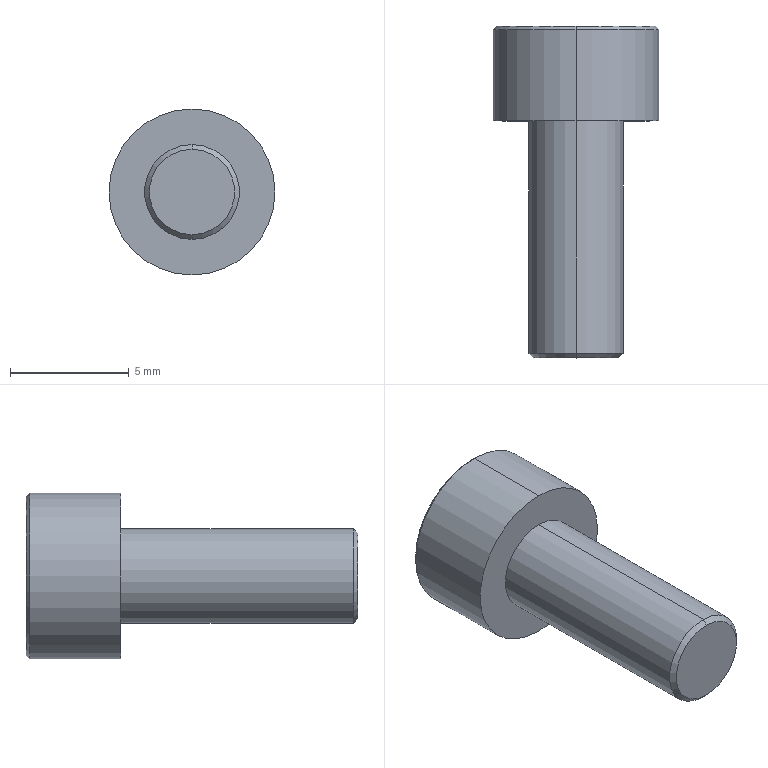Part | STEP file | Guide wheel mechanism revised.sldasm-Part-511 | 1 solid | 32 faces | box 7 x 14 x 7 mm | volume 260.581 mm3 | plane 15 | cone 13 | cylinder 4 | commonest cylinder face diameters 4 x2 7 x2
STEP:
#1=CARTESIAN_POINT('',(0.,-13.8,2.));
#2=VERTEX_POINT('',#1);
#3=CARTESIAN_POINT('',(0.,-13.8,-2.));
#4=VERTEX_POINT('',#3);
#5=CARTESIAN_POINT('',(0.,-13.8,0.));
#6=DIRECTION('',(0.,1.,0.));
#7=DIRECTION('',(0.,0.,1.));
#8=AXIS2_PLACEMENT_3D('',#5,#6,#7);
#9=CIRCLE('',#8,2.);
#10=EDGE_CURVE('',#2,#4,#9,.T.);
#11=ORIENTED_EDGE('',*,*,#10,.T.);
#12=CARTESIAN_POINT('',(0.,-4.,-2.));
#13=VERTEX_POINT('',#12);
#14=CARTESIAN_POINT('',(0.,-14.7,-2.));
#15=DIRECTION('',(0.,1.,0.));
#16=VECTOR('',#15,1000.);
#17=LINE('',#14,#16);
#18=EDGE_CURVE('',#4,#13,#17,.T.);
#19=ORIENTED_EDGE('',*,*,#18,.T.);
#20=CARTESIAN_POINT('',(0.,-4.,2.));
#21=VERTEX_POINT('',#20);
#22=CARTESIAN_POINT('',(0.,-4.,0.));
#23=DIRECTION('',(0.,-1.,0.));
#24=DIRECTION('',(0.,0.,1.));
#25=AXIS2_PLACEMENT_3D('',#22,#23,#24);
#26=CIRCLE('',#25,2.);
#27=EDGE_CURVE('',#13,#21,#26,.T.);
#28=ORIENTED_EDGE('',*,*,#27,.T.);
#29=CARTESIAN_POINT('',(0.,-14.7,2.));
#30=DIRECTION('',(0.,1.,0.));
#31=VECTOR('',#30,1000.);
#32=LINE('',#29,#31);
#33=EDGE_CURVE('',#2,#21,#32,.T.);
#34=ORIENTED_EDGE('',*,*,#33,.F.);
#35=EDGE_LOOP('',(#11,#19,#28,#34));
#36=FACE_OUTER_BOUND('',#35,.T.);
#37=CARTESIAN_POINT('',(0.,-14.7,0.));
#38=DIRECTION('',(0.,1.,0.));
#39=DIRECTION('',(0.,0.,1.));
#40=AXIS2_PLACEMENT_3D('',#37,#38,#39);
#41=CYLINDRICAL_SURFACE('',#40,2.);
#42=ADVANCED_FACE('',(#36),#41,.T.);
#43=CARTESIAN_POINT('',(0.,-14.,1.8));
#44=VERTEX_POINT('',#43);
#45=CARTESIAN_POINT('',(0.,-14.,-1.8));
#46=VERTEX_POINT('',#45);
#47=CARTESIAN_POINT('',(0.,-14.,0.));
#48=DIRECTION('',(0.,1.,0.));
#49=DIRECTION('',(0.,0.,1.));
#50=AXIS2_PLACEMENT_3D('',#47,#48,#49);
#51=CIRCLE('',#50,1.8);
#52=EDGE_CURVE('',#44,#46,#51,.T.);
#53=ORIENTED_EDGE('',*,*,#52,.T.);
#54=CARTESIAN_POINT('',(0.,-13.8,-2.));
#55=DIRECTION('',(0.,0.7071,-0.7071));
#56=VECTOR('',#55,1000.);
#57=LINE('',#54,#56);
#58=EDGE_CURVE('',#46,#4,#57,.T.);
#59=ORIENTED_EDGE('',*,*,#58,.T.);
#60=ORIENTED_EDGE('',*,*,#10,.F.);
#61=CARTESIAN_POINT('',(0.,-13.8,2.));
#62=DIRECTION('',(0.,0.7071,0.7071));
#63=VECTOR('',#62,1000.);
#64=LINE('',#61,#63);
#65=EDGE_CURVE('',#44,#2,#64,.T.);
#66=ORIENTED_EDGE('',*,*,#65,.F.);
#67=EDGE_LOOP('',(#53,#59,#60,#66));
#68=FACE_OUTER_BOUND('',#67,.T.);
#69=CARTESIAN_POINT('',(0.,-13.8,0.));
#70=DIRECTION('',(0.,1.,0.));
#71=DIRECTION('',(0.,0.,1.));
#72=AXIS2_PLACEMENT_3D('',#69,#70,#71);
#73=CONICAL_SURFACE('',#72,2.,0.7854);
#74=ADVANCED_FACE('',(#68),#73,.T.);
#75=CARTESIAN_POINT('',(0.,-4.,3.5));
#76=VERTEX_POINT('',#75);
#77=CARTESIAN_POINT('',(0.,-4.,-3.5));
#78=VERTEX_POINT('',#77);
#79=CARTESIAN_POINT('',(0.,-4.,0.));
#80=DIRECTION('',(0.,1.,0.));
#81=DIRECTION('',(0.,0.,1.));
#82=AXIS2_PLACEMENT_3D('',#79,#80,#81);
#83=CIRCLE('',#82,3.5);
#84=EDGE_CURVE('',#76,#78,#83,.T.);
#85=ORIENTED_EDGE('',*,*,#84,.T.);
#86=CARTESIAN_POINT('',(0.,-0.15,-3.5));
#87=VERTEX_POINT('',#86);
#88=CARTESIAN_POINT('',(0.,-14.7,-3.5));
#89=DIRECTION('',(0.,1.,0.));
#90=VECTOR('',#89,1000.);
#91=LINE('',#88,#90);
#92=EDGE_CURVE('',#78,#87,#91,.T.);
#93=ORIENTED_EDGE('',*,*,#92,.T.);
#94=CARTESIAN_POINT('',(0.,-0.15,3.5));
#95=VERTEX_POINT('',#94);
#96=CARTESIAN_POINT('',(0.,-0.15,0.));
#97=DIRECTION('',(0.,-1.,0.));
#98=DIRECTION('',(0.,0.,1.));
#99=AXIS2_PLACEMENT_3D('',#96,#97,#98);
#100=CIRCLE('',#99,3.5);
#101=EDGE_CURVE('',#87,#95,#100,.T.);
#102=ORIENTED_EDGE('',*,*,#101,.T.);
#103=CARTESIAN_POINT('',(0.,-14.7,3.5));
#104=DIRECTION('',(0.,1.,0.));
#105=VECTOR('',#104,1000.);
#106=LINE('',#103,#105);
#107=EDGE_CURVE('',#76,#95,#106,.T.);
#108=ORIENTED_EDGE('',*,*,#107,.F.);
#109=EDGE_LOOP('',(#85,#93,#102,#108));
#110=FACE_OUTER_BOUND('',#109,.T.);
#111=CARTESIAN_POINT('',(0.,-14.7,0.));
#112=DIRECTION('',(0.,1.,0.));
#113=DIRECTION('',(0.,0.,1.));
#114=AXIS2_PLACEMENT_3D('',#111,#112,#113);
#115=CYLINDRICAL_SURFACE('',#114,3.5);
#116=ADVANCED_FACE('',(#110),#115,.T.);
#117=CARTESIAN_POINT('',(0.,0.,-3.35));
#118=VERTEX_POINT('',#117);
#119=CARTESIAN_POINT('',(0.,0.,3.35));
#120=VERTEX_POINT('',#119);
#121=CARTESIAN_POINT('',(0.,0.,0.));
#122=DIRECTION('',(0.,-1.,0.));
#123=DIRECTION('',(0.,0.,-1.));
#124=AXIS2_PLACEMENT_3D('',#121,#122,#123);
#125=CIRCLE('',#124,3.35);
#126=EDGE_CURVE('',#118,#120,#125,.T.);
#127=ORIENTED_EDGE('',*,*,#126,.T.);
#128=CARTESIAN_POINT('',(0.,-0.15,3.5));
#129=DIRECTION('',(0.,-0.7071,0.7071));
#130=VECTOR('',#129,1000.);
#131=LINE('',#128,#130);
#132=EDGE_CURVE('',#120,#95,#131,.T.);
#133=ORIENTED_EDGE('',*,*,#132,.T.);
#134=ORIENTED_EDGE('',*,*,#101,.F.);
#135=CARTESIAN_POINT('',(0.,-0.15,-3.5));
#136=DIRECTION('',(0.,-0.7071,-0.7071));
#137=VECTOR('',#136,1000.);
#138=LINE('',#135,#137);
#139=EDGE_CURVE('',#118,#87,#138,.T.);
#140=ORIENTED_EDGE('',*,*,#139,.F.);
#141=EDGE_LOOP('',(#127,#133,#134,#140));
#142=FACE_OUTER_BOUND('',#141,.T.);
#143=CARTESIAN_POINT('',(0.,-0.15,0.));
#144=DIRECTION('',(0.,-1.,0.));
#145=DIRECTION('',(0.,0.,-1.));
#146=AXIS2_PLACEMENT_3D('',#143,#144,#145);
#147=CONICAL_SURFACE('',#146,3.5,0.7854);
#148=ADVANCED_FACE('',(#142),#147,.T.);
#149=CARTESIAN_POINT('',(0.,-0.133,1.49));
#150=VERTEX_POINT('',#149);
#151=CARTESIAN_POINT('',(0.86,0.,1.49));
#152=VERTEX_POINT('',#151);
#153=CARTESIAN_POINT('',(0.,-0.133,1.49));
#154=CARTESIAN_POINT('',(0.2919,-0.133,1.49));
#155=CARTESIAN_POINT('',(0.5793,-0.08102,1.49));
#156=CARTESIAN_POINT('',(0.86,0.,1.49));
#157=B_SPLINE_CURVE_WITH_KNOTS('',3,(#153,#154,#155,#156),.UNSPECIFIED.,.F.,.F.,(4,4),(0.0008702,0.001737),.UNSPECIFIED.);
#158=EDGE_CURVE('',#150,#152,#157,.T.);
#159=ORIENTED_EDGE('',*,*,#158,.F.);
#160=CARTESIAN_POINT('',(0.,0.,1.72));
#161=VERTEX_POINT('',#160);
#162=CARTESIAN_POINT('',(0.,0.,1.72));
#163=DIRECTION('',(0.,0.5,0.866));
#164=VECTOR('',#163,1000.);
#165=LINE('',#162,#164);
#166=EDGE_CURVE('',#150,#161,#165,.T.);
#167=ORIENTED_EDGE('',*,*,#166,.T.);
#168=CARTESIAN_POINT('',(0.,0.,0.));
#169=DIRECTION('',(0.,-1.,0.));
#170=DIRECTION('',(0.,0.,1.));
#171=AXIS2_PLACEMENT_3D('',#168,#169,#170);
#172=CIRCLE('',#171,1.72);
#173=EDGE_CURVE('',#152,#161,#172,.T.);
#174=ORIENTED_EDGE('',*,*,#173,.F.);
#175=EDGE_LOOP('',(#159,#167,#174));
#176=FACE_OUTER_BOUND('',#175,.T.);
#177=CARTESIAN_POINT('',(0.,0.,0.));
#178=DIRECTION('',(0.,1.,0.));
#179=DIRECTION('',(0.,0.,1.));
#180=AXIS2_PLACEMENT_3D('',#177,#178,#179);
#181=CONICAL_SURFACE('',#180,1.72,1.047);
#182=ADVANCED_FACE('',(#176),#181,.F.);
#183=CARTESIAN_POINT('',(0.,-2.993,0.));
#184=VERTEX_POINT('',#183);
#185=CARTESIAN_POINT('',(0.,-2.,1.72));
#186=VERTEX_POINT('',#185);
#187=CARTESIAN_POINT('',(0.,-2.,1.72));
#188=DIRECTION('',(0.,0.5,0.866));
#189=VECTOR('',#188,1000.);
#190=LINE('',#187,#189);
#191=EDGE_CURVE('',#184,#186,#190,.T.);
#192=ORIENTED_EDGE('',*,*,#191,.F.);
#193=CARTESIAN_POINT('',(0.,-2.,-1.72));
#194=VERTEX_POINT('',#193);
#195=CARTESIAN_POINT('',(0.,-2.,-1.72));
#196=DIRECTION('',(0.,0.5,-0.866));
#197=VECTOR('',#196,1000.);
#198=LINE('',#195,#197);
#199=EDGE_CURVE('',#184,#194,#198,.T.);
#200=ORIENTED_EDGE('',*,*,#199,.T.);
#201=CARTESIAN_POINT('',(-0.86,-2.,-1.49));
#202=VERTEX_POINT('',#201);
#203=CARTESIAN_POINT('',(0.,-2.,0.));
#204=DIRECTION('',(0.,-1.,0.));
#205=DIRECTION('',(0.,0.,1.));
#206=AXIS2_PLACEMENT_3D('',#203,#204,#205);
#207=CIRCLE('',#206,1.72);
#208=EDGE_CURVE('',#202,#194,#207,.T.);
#209=ORIENTED_EDGE('',*,*,#208,.F.);
#210=CARTESIAN_POINT('',(-1.72,-2.,0.));
#211=VERTEX_POINT('',#210);
#212=CARTESIAN_POINT('',(0.,-2.,0.));
#213=DIRECTION('',(0.,-1.,0.));
#214=DIRECTION('',(0.,0.,1.));
#215=AXIS2_PLACEMENT_3D('',#212,#213,#214);
#216=CIRCLE('',#215,1.72);
#217=EDGE_CURVE('',#211,#202,#216,.T.);
#218=ORIENTED_EDGE('',*,*,#217,.F.);
#219=CARTESIAN_POINT('',(-0.86,-2.,1.49));
#220=VERTEX_POINT('',#219);
#221=CARTESIAN_POINT('',(0.,-2.,0.));
#222=DIRECTION('',(0.,-1.,0.));
#223=DIRECTION('',(0.,0.,1.));
#224=AXIS2_PLACEMENT_3D('',#221,#222,#223);
#225=CIRCLE('',#224,1.72);
#226=EDGE_CURVE('',#220,#211,#225,.T.);
#227=ORIENTED_EDGE('',*,*,#226,.F.);
#228=CARTESIAN_POINT('',(0.,-2.,0.));
#229=DIRECTION('',(0.,1.,0.));
#230=DIRECTION('',(0.,0.,1.));
#231=AXIS2_PLACEMENT_3D('',#228,#229,#230);
#232=CIRCLE('',#231,1.72);
#233=EDGE_CURVE('',#220,#186,#232,.T.);
#234=ORIENTED_EDGE('',*,*,#233,.T.);
#235=EDGE_LOOP('',(#192,#200,#209,#218,#227,#234));
#236=FACE_OUTER_BOUND('',#235,.T.);
#237=CARTESIAN_POINT('',(0.,-2.,0.));
#238=DIRECTION('',(0.,1.,0.));
#239=DIRECTION('',(0.,0.,1.));
#240=AXIS2_PLACEMENT_3D('',#237,#238,#239);
#241=CONICAL_SURFACE('',#240,1.72,1.047);
#242=ADVANCED_FACE('',(#236),#241,.F.);
#243=ORIENTED_EDGE('',*,*,#18,.F.);
#244=CARTESIAN_POINT('',(0.,-13.8,0.));
#245=DIRECTION('',(0.,1.,0.));
#246=DIRECTION('',(0.,0.,1.));
#247=AXIS2_PLACEMENT_3D('',#244,#245,#246);
#248=CIRCLE('',#247,2.);
#249=EDGE_CURVE('',#4,#2,#248,.T.);
#250=ORIENTED_EDGE('',*,*,#249,.T.);
#251=ORIENTED_EDGE('',*,*,#33,.T.);
#252=CARTESIAN_POINT('',(0.,-4.,0.));
#253=DIRECTION('',(0.,-1.,0.));
#254=DIRECTION('',(0.,0.,1.));
#255=AXIS2_PLACEMENT_3D('',#252,#253,#254);
#256=CIRCLE('',#255,2.);
#257=EDGE_CURVE('',#21,#13,#256,.T.);
#258=ORIENTED_EDGE('',*,*,#257,.T.);
#259=EDGE_LOOP('',(#243,#250,#251,#258));
#260=FACE_OUTER_BOUND('',#259,.T.);
#261=CARTESIAN_POINT('',(0.,-14.7,0.));
#262=DIRECTION('',(0.,1.,0.));
#263=DIRECTION('',(0.,0.,1.));
#264=AXIS2_PLACEMENT_3D('',#261,#262,#263);
#265=CYLINDRICAL_SURFACE('',#264,2.);
#266=ADVANCED_FACE('',(#260),#265,.T.);
#267=ORIENTED_EDGE('',*,*,#257,.F.);
#268=ORIENTED_EDGE('',*,*,#27,.F.);
#269=EDGE_LOOP('',(#267,#268));
#270=FACE_BOUND('',#269,.T.);
#271=ORIENTED_EDGE('',*,*,#84,.F.);
#272=CARTESIAN_POINT('',(0.,-4.,0.));
#273=DIRECTION('',(0.,1.,0.));
#274=DIRECTION('',(0.,0.,1.));
#275=AXIS2_PLACEMENT_3D('',#272,#273,#274);
#276=CIRCLE('',#275,3.5);
#277=EDGE_CURVE('',#78,#76,#276,.T.);
#278=ORIENTED_EDGE('',*,*,#277,.F.);
#279=EDGE_LOOP('',(#271,#278));
#280=FACE_OUTER_BOUND('',#279,.T.);
#281=CARTESIAN_POINT('',(0.,-4.,0.));
#282=DIRECTION('',(0.,1.,0.));
#283=DIRECTION('',(0.,0.,1.));
#284=AXIS2_PLACEMENT_3D('',#281,#282,#283);
#285=PLANE('',#284);
#286=ADVANCED_FACE('',(#270,#280),#285,.F.);
#287=ORIENTED_EDGE('',*,*,#58,.F.);
#288=CARTESIAN_POINT('',(0.,-14.,0.));
#289=DIRECTION('',(0.,1.,0.));
#290=DIRECTION('',(0.,0.,1.));
#291=AXIS2_PLACEMENT_3D('',#288,#289,#290);
#292=CIRCLE('',#291,1.8);
#293=EDGE_CURVE('',#46,#44,#292,.T.);
#294=ORIENTED_EDGE('',*,*,#293,.T.);
#295=ORIENTED_EDGE('',*,*,#65,.T.);
#296=ORIENTED_EDGE('',*,*,#249,.F.);
#297=EDGE_LOOP('',(#287,#294,#295,#296));
#298=FACE_OUTER_BOUND('',#297,.T.);
#299=CARTESIAN_POINT('',(0.,-13.8,0.));
#300=DIRECTION('',(0.,1.,0.));
#301=DIRECTION('',(0.,0.,1.));
#302=AXIS2_PLACEMENT_3D('',#299,#300,#301);
#303=CONICAL_SURFACE('',#302,2.,0.7854);
#304=ADVANCED_FACE('',(#298),#303,.T.);
#305=ORIENTED_EDGE('',*,*,#92,.F.);
#306=ORIENTED_EDGE('',*,*,#277,.T.);
#307=ORIENTED_EDGE('',*,*,#107,.T.);
#308=CARTESIAN_POINT('',(0.,-0.15,0.));
#309=DIRECTION('',(0.,-1.,0.));
#310=DIRECTION('',(0.,0.,1.));
#311=AXIS2_PLACEMENT_3D('',#308,#309,#310);
#312=CIRCLE('',#311,3.5);
#313=EDGE_CURVE('',#95,#87,#312,.T.);
#314=ORIENTED_EDGE('',*,*,#313,.T.);
#315=EDGE_LOOP('',(#305,#306,#307,#314));
#316=FACE_OUTER_BOUND('',#315,.T.);
#317=CARTESIAN_POINT('',(0.,-14.7,0.));
#318=DIRECTION('',(0.,1.,0.));
#319=DIRECTION('',(0.,0.,1.));
#320=AXIS2_PLACEMENT_3D('',#317,#318,#319);
#321=CYLINDRICAL_SURFACE('',#320,3.5);
#322=ADVANCED_FACE('',(#316),#321,.T.);
#323=ORIENTED_EDGE('',*,*,#52,.F.);
#324=ORIENTED_EDGE('',*,*,#293,.F.);
#325=EDGE_LOOP('',(#323,#324));
#326=FACE_OUTER_BOUND('',#325,.T.);
#327=CARTESIAN_POINT('',(0.,-14.,0.));
#328=DIRECTION('',(0.,1.,0.));
#329=DIRECTION('',(0.,0.,1.));
#330=AXIS2_PLACEMENT_3D('',#327,#328,#329);
#331=PLANE('',#330);
#332=ADVANCED_FACE('',(#326),#331,.F.);
#333=ORIENTED_EDGE('',*,*,#132,.F.);
#334=CARTESIAN_POINT('',(0.,0.,0.));
#335=DIRECTION('',(0.,-1.,0.));
#336=DIRECTION('',(0.,0.,-1.));
#337=AXIS2_PLACEMENT_3D('',#334,#335,#336);
#338=CIRCLE('',#337,3.35);
#339=EDGE_CURVE('',#120,#118,#338,.T.);
#340=ORIENTED_EDGE('',*,*,#339,.T.);
#341=ORIENTED_EDGE('',*,*,#139,.T.);
#342=ORIENTED_EDGE('',*,*,#313,.F.);
#343=EDGE_LOOP('',(#333,#340,#341,#342));
#344=FACE_OUTER_BOUND('',#343,.T.);
#345=CARTESIAN_POINT('',(0.,-0.15,0.));
#346=DIRECTION('',(0.,-1.,0.));
#347=DIRECTION('',(0.,0.,-1.));
#348=AXIS2_PLACEMENT_3D('',#345,#346,#347);
#349=CONICAL_SURFACE('',#348,3.5,0.7854);
#350=ADVANCED_FACE('',(#344),#349,.T.);
#351=CARTESIAN_POINT('',(-0.86,0.,-1.49));
#352=VERTEX_POINT('',#351);
#353=CARTESIAN_POINT('',(0.86,0.,-1.49));
#354=VERTEX_POINT('',#353);
#355=CARTESIAN_POINT('',(0.,0.,0.));
#356=DIRECTION('',(0.,-1.,0.));
#357=DIRECTION('',(0.,0.,1.));
#358=AXIS2_PLACEMENT_3D('',#355,#356,#357);
#359=CIRCLE('',#358,1.72);
#360=EDGE_CURVE('',#352,#354,#359,.T.);
#361=ORIENTED_EDGE('',*,*,#360,.T.);
#362=CARTESIAN_POINT('',(1.72,0.,0.));
#363=VERTEX_POINT('',#362);
#364=CARTESIAN_POINT('',(0.,0.,0.));
#365=DIRECTION('',(0.,-1.,0.));
#366=DIRECTION('',(0.,0.,1.));
#367=AXIS2_PLACEMENT_3D('',#364,#365,#366);
#368=CIRCLE('',#367,1.72);
#369=EDGE_CURVE('',#354,#363,#368,.T.);
#370=ORIENTED_EDGE('',*,*,#369,.T.);
#371=CARTESIAN_POINT('',(0.,0.,0.));
#372=DIRECTION('',(0.,-1.,0.));
#373=DIRECTION('',(0.,0.,1.));
#374=AXIS2_PLACEMENT_3D('',#371,#372,#373);
#375=CIRCLE('',#374,1.72);
#376=EDGE_CURVE('',#363,#152,#375,.T.);
#377=ORIENTED_EDGE('',*,*,#376,.T.);
#378=ORIENTED_EDGE('',*,*,#173,.T.);
#379=CARTESIAN_POINT('',(-0.86,0.,1.49));
#380=VERTEX_POINT('',#379);
#381=CARTESIAN_POINT('',(0.,0.,0.));
#382=DIRECTION('',(0.,-1.,0.));
#383=DIRECTION('',(0.,0.,1.));
#384=AXIS2_PLACEMENT_3D('',#381,#382,#383);
#385=CIRCLE('',#384,1.72);
#386=EDGE_CURVE('',#161,#380,#385,.T.);
#387=ORIENTED_EDGE('',*,*,#386,.T.);
#388=CARTESIAN_POINT('',(-1.72,0.,0.));
#389=VERTEX_POINT('',#388);
#390=CARTESIAN_POINT('',(0.,0.,0.));
#391=DIRECTION('',(0.,-1.,0.));
#392=DIRECTION('',(0.,0.,1.));
#393=AXIS2_PLACEMENT_3D('',#390,#391,#392);
#394=CIRCLE('',#393,1.72);
#395=EDGE_CURVE('',#380,#389,#394,.T.);
#396=ORIENTED_EDGE('',*,*,#395,.T.);
#397=CARTESIAN_POINT('',(0.,0.,0.));
#398=DIRECTION('',(0.,-1.,0.));
#399=DIRECTION('',(0.,0.,1.));
#400=AXIS2_PLACEMENT_3D('',#397,#398,#399);
#401=CIRCLE('',#400,1.72);
#402=EDGE_CURVE('',#389,#352,#401,.T.);
#403=ORIENTED_EDGE('',*,*,#402,.T.);
#404=EDGE_LOOP('',(#361,#370,#377,#378,#387,#396,#403));
#405=FACE_BOUND('',#404,.T.);
#406=ORIENTED_EDGE('',*,*,#126,.F.);
#407=ORIENTED_EDGE('',*,*,#339,.F.);
#408=EDGE_LOOP('',(#406,#407));
#409=FACE_OUTER_BOUND('',#408,.T.);
#410=CARTESIAN_POINT('',(0.,0.,0.));
#411=DIRECTION('',(0.,1.,0.));
#412=DIRECTION('',(0.,0.,1.));
#413=AXIS2_PLACEMENT_3D('',#410,#411,#412);
#414=PLANE('',#413);
#415=ADVANCED_FACE('',(#405,#409),#414,.T.);
#416=CARTESIAN_POINT('',(1.72,0.,0.));
#417=CARTESIAN_POINT('',(1.58,-0.08107,-0.2432));
#418=CARTESIAN_POINT('',(1.437,-0.1329,-0.4901));
#419=CARTESIAN_POINT('',(1.145,-0.1332,-0.9966));
#420=CARTESIAN_POINT('',(1.001,-0.08117,-1.246));
#421=CARTESIAN_POINT('',(0.86,0.,-1.49));
#422=B_SPLINE_CURVE_WITH_KNOTS('',3,(#416,#417,#418,#419,#420,#421),.UNSPECIFIED.,.F.,.F.,(4,2,4),(0.,0.0008686,0.001737),.UNSPECIFIED.);
#423=EDGE_CURVE('',#363,#354,#422,.T.);
#424=ORIENTED_EDGE('',*,*,#423,.F.);
#425=ORIENTED_EDGE('',*,*,#369,.F.);
#426=EDGE_LOOP('',(#424,#425));
#427=FACE_OUTER_BOUND('',#426,.T.);
#428=CARTESIAN_POINT('',(0.,0.,0.));
#429=DIRECTION('',(0.,1.,0.));
#430=DIRECTION('',(0.,0.,1.));
#431=AXIS2_PLACEMENT_3D('',#428,#429,#430);
#432=CONICAL_SURFACE('',#431,1.72,1.047);
#433=ADVANCED_FACE('',(#427),#432,.F.);
#434=CARTESIAN_POINT('',(0.86,0.,-1.49));
#435=CARTESIAN_POINT('',(0.5792,-0.08107,-1.49));
#436=CARTESIAN_POINT('',(0.2941,-0.1329,-1.49));
#437=CARTESIAN_POINT('',(-0.2908,-0.1332,-1.49));
#438=CARTESIAN_POINT('',(-0.5788,-0.08117,-1.49));
#439=CARTESIAN_POINT('',(-0.86,0.,-1.49));
#440=B_SPLINE_CURVE_WITH_KNOTS('',3,(#434,#435,#436,#437,#438,#439),.UNSPECIFIED.,.F.,.F.,(4,2,4),(0.,0.0008686,0.001737),.UNSPECIFIED.);
#441=EDGE_CURVE('',#354,#352,#440,.T.);
#442=ORIENTED_EDGE('',*,*,#441,.F.);
#443=ORIENTED_EDGE('',*,*,#360,.F.);
#444=EDGE_LOOP('',(#442,#443));
#445=FACE_OUTER_BOUND('',#444,.T.);
#446=CARTESIAN_POINT('',(0.,0.,0.));
#447=DIRECTION('',(0.,1.,0.));
#448=DIRECTION('',(0.,0.,1.));
#449=AXIS2_PLACEMENT_3D('',#446,#447,#448);
#450=CONICAL_SURFACE('',#449,1.72,1.047);
#451=ADVANCED_FACE('',(#445),#450,.F.);
#452=CARTESIAN_POINT('',(-0.86,0.,-1.49));
#453=CARTESIAN_POINT('',(-1.,-0.08107,-1.246));
#454=CARTESIAN_POINT('',(-1.143,-0.1329,-0.9995));
#455=CARTESIAN_POINT('',(-1.435,-0.1332,-0.4929));
#456=CARTESIAN_POINT('',(-1.579,-0.08117,-0.2435));
#457=CARTESIAN_POINT('',(-1.72,0.,0.));
#458=B_SPLINE_CURVE_WITH_KNOTS('',3,(#452,#453,#454,#455,#456,#457),.UNSPECIFIED.,.F.,.F.,(4,2,4),(0.,0.0008686,0.001737),.UNSPECIFIED.);
#459=EDGE_CURVE('',#352,#389,#458,.T.);
#460=ORIENTED_EDGE('',*,*,#459,.F.);
#461=ORIENTED_EDGE('',*,*,#402,.F.);
#462=EDGE_LOOP('',(#460,#461));
#463=FACE_OUTER_BOUND('',#462,.T.);
#464=CARTESIAN_POINT('',(0.,0.,0.));
#465=DIRECTION('',(0.,1.,0.));
#466=DIRECTION('',(0.,0.,1.));
#467=AXIS2_PLACEMENT_3D('',#464,#465,#466);
#468=CONICAL_SURFACE('',#467,1.72,1.047);
#469=ADVANCED_FACE('',(#463),#468,.F.);
#470=CARTESIAN_POINT('',(-1.72,0.,0.));
#471=CARTESIAN_POINT('',(-1.58,-0.08107,0.2432));
#472=CARTESIAN_POINT('',(-1.437,-0.1329,0.4901));
#473=CARTESIAN_POINT('',(-1.145,-0.1332,0.9966));
#474=CARTESIAN_POINT('',(-1.001,-0.08117,1.246));
#475=CARTESIAN_POINT('',(-0.86,0.,1.49));
#476=B_SPLINE_CURVE_WITH_KNOTS('',3,(#470,#471,#472,#473,#474,#475),.UNSPECIFIED.,.F.,.F.,(4,2,4),(0.,0.0008686,0.001737),.UNSPECIFIED.);
#477=EDGE_CURVE('',#389,#380,#476,.T.);
#478=ORIENTED_EDGE('',*,*,#477,.F.);
#479=ORIENTED_EDGE('',*,*,#395,.F.);
#480=EDGE_LOOP('',(#478,#479));
#481=FACE_OUTER_BOUND('',#480,.T.);
#482=CARTESIAN_POINT('',(0.,0.,0.));
#483=DIRECTION('',(0.,1.,0.));
#484=DIRECTION('',(0.,0.,1.));
#485=AXIS2_PLACEMENT_3D('',#482,#483,#484);
#486=CONICAL_SURFACE('',#485,1.72,1.047);
#487=ADVANCED_FACE('',(#481),#486,.F.);
#488=ORIENTED_EDGE('',*,*,#166,.F.);
#489=CARTESIAN_POINT('',(-0.86,0.,1.49));
#490=CARTESIAN_POINT('',(-0.5786,-0.08122,1.49));
#491=CARTESIAN_POINT('',(-0.293,-0.133,1.49));
#492=CARTESIAN_POINT('',(0.,-0.133,1.49));
#493=B_SPLINE_CURVE_WITH_KNOTS('',3,(#489,#490,#491,#492),.UNSPECIFIED.,.F.,.F.,(4,4),(0.,0.0008702),.UNSPECIFIED.);
#494=EDGE_CURVE('',#380,#150,#493,.T.);
#495=ORIENTED_EDGE('',*,*,#494,.F.);
#496=ORIENTED_EDGE('',*,*,#386,.F.);
#497=EDGE_LOOP('',(#488,#495,#496));
#498=FACE_OUTER_BOUND('',#497,.T.);
#499=CARTESIAN_POINT('',(0.,0.,0.));
#500=DIRECTION('',(0.,1.,0.));
#501=DIRECTION('',(0.,0.,1.));
#502=AXIS2_PLACEMENT_3D('',#499,#500,#501);
#503=CONICAL_SURFACE('',#502,1.72,1.047);
#504=ADVANCED_FACE('',(#498),#503,.F.);
#505=CARTESIAN_POINT('',(0.86,0.,1.49));
#506=CARTESIAN_POINT('',(1.,-0.08107,1.246));
#507=CARTESIAN_POINT('',(1.143,-0.1329,0.9995));
#508=CARTESIAN_POINT('',(1.435,-0.1332,0.4929));
#509=CARTESIAN_POINT('',(1.579,-0.08117,0.2435));
#510=CARTESIAN_POINT('',(1.72,0.,0.));
#511=B_SPLINE_CURVE_WITH_KNOTS('',3,(#505,#506,#507,#508,#509,#510),.UNSPECIFIED.,.F.,.F.,(4,2,4),(0.,0.0008686,0.001737),.UNSPECIFIED.);
#512=EDGE_CURVE('',#152,#363,#511,.T.);
#513=ORIENTED_EDGE('',*,*,#512,.F.);
#514=ORIENTED_EDGE('',*,*,#376,.F.);
#515=EDGE_LOOP('',(#513,#514));
#516=FACE_OUTER_BOUND('',#515,.T.);
#517=CARTESIAN_POINT('',(0.,0.,0.));
#518=DIRECTION('',(0.,1.,0.));
#519=DIRECTION('',(0.,0.,1.));
#520=AXIS2_PLACEMENT_3D('',#517,#518,#519);
#521=CONICAL_SURFACE('',#520,1.72,1.047);
#522=ADVANCED_FACE('',(#516),#521,.F.);
#523=ORIENTED_EDGE('',*,*,#423,.T.);
#524=CARTESIAN_POINT('',(0.86,-2.,-1.49));
#525=VERTEX_POINT('',#524);
#526=CARTESIAN_POINT('',(0.86,0.,-1.49));
#527=DIRECTION('',(0.,1.,0.));
#528=VECTOR('',#527,1000.);
#529=LINE('',#526,#528);
#530=EDGE_CURVE('',#525,#354,#529,.T.);
#531=ORIENTED_EDGE('',*,*,#530,.F.);
#532=CARTESIAN_POINT('',(1.72,-2.,0.));
#533=VERTEX_POINT('',#532);
#534=CARTESIAN_POINT('',(0.86,-2.,-1.49));
#535=DIRECTION('',(0.5,0.,0.866));
#536=VECTOR('',#535,1000.);
#537=LINE('',#534,#536);
#538=EDGE_CURVE('',#525,#533,#537,.T.);
#539=ORIENTED_EDGE('',*,*,#538,.T.);
#540=CARTESIAN_POINT('',(1.72,0.,0.));
#541=DIRECTION('',(0.,-1.,0.));
#542=VECTOR('',#541,1000.);
#543=LINE('',#540,#542);
#544=EDGE_CURVE('',#363,#533,#543,.T.);
#545=ORIENTED_EDGE('',*,*,#544,.F.);
#546=EDGE_LOOP('',(#523,#531,#539,#545));
#547=FACE_OUTER_BOUND('',#546,.T.);
#548=CARTESIAN_POINT('',(1.72,0.,0.));
#549=DIRECTION('',(0.866,0.,-0.5));
#550=DIRECTION('',(-0.5,0.,-0.866));
#551=AXIS2_PLACEMENT_3D('',#548,#549,#550);
#552=PLANE('',#551);
#553=ADVANCED_FACE('',(#547),#552,.F.);
#554=ORIENTED_EDGE('',*,*,#441,.T.);
#555=CARTESIAN_POINT('',(-0.86,0.,-1.49));
#556=DIRECTION('',(0.,1.,0.));
#557=VECTOR('',#556,1000.);
#558=LINE('',#555,#557);
#559=EDGE_CURVE('',#202,#352,#558,.T.);
#560=ORIENTED_EDGE('',*,*,#559,.F.);
#561=CARTESIAN_POINT('',(0.,-2.,-1.49));
#562=DIRECTION('',(1.,0.,0.));
#563=VECTOR('',#562,1000.);
#564=LINE('',#561,#563);
#565=EDGE_CURVE('',#202,#525,#564,.T.);
#566=ORIENTED_EDGE('',*,*,#565,.T.);
#567=ORIENTED_EDGE('',*,*,#530,.T.);
#568=EDGE_LOOP('',(#554,#560,#566,#567));
#569=FACE_OUTER_BOUND('',#568,.T.);
#570=CARTESIAN_POINT('',(0.86,0.,-1.49));
#571=DIRECTION('',(0.,0.,-1.));
#572=DIRECTION('',(-1.,0.,0.));
#573=AXIS2_PLACEMENT_3D('',#570,#571,#572);
#574=PLANE('',#573);
#575=ADVANCED_FACE('',(#569),#574,.F.);
#576=ORIENTED_EDGE('',*,*,#459,.T.);
#577=CARTESIAN_POINT('',(-1.72,0.,0.));
#578=DIRECTION('',(0.,1.,0.));
#579=VECTOR('',#578,1000.);
#580=LINE('',#577,#579);
#581=EDGE_CURVE('',#211,#389,#580,.T.);
#582=ORIENTED_EDGE('',*,*,#581,.F.);
#583=CARTESIAN_POINT('',(-1.72,-2.,0.));
#584=DIRECTION('',(0.5,0.,-0.866));
#585=VECTOR('',#584,1000.);
#586=LINE('',#583,#585);
#587=EDGE_CURVE('',#211,#202,#586,.T.);
#588=ORIENTED_EDGE('',*,*,#587,.T.);
#589=ORIENTED_EDGE('',*,*,#559,.T.);
#590=EDGE_LOOP('',(#576,#582,#588,#589));
#591=FACE_OUTER_BOUND('',#590,.T.);
#592=CARTESIAN_POINT('',(-0.86,0.,-1.49));
#593=DIRECTION('',(-0.866,0.,-0.5));
#594=DIRECTION('',(-0.5,0.,0.866));
#595=AXIS2_PLACEMENT_3D('',#592,#593,#594);
#596=PLANE('',#595);
#597=ADVANCED_FACE('',(#591),#596,.F.);
#598=ORIENTED_EDGE('',*,*,#477,.T.);
#599=CARTESIAN_POINT('',(-0.86,0.,1.49));
#600=DIRECTION('',(0.,1.,0.));
#601=VECTOR('',#600,1000.);
#602=LINE('',#599,#601);
#603=EDGE_CURVE('',#220,#380,#602,.T.);
#604=ORIENTED_EDGE('',*,*,#603,.F.);
#605=CARTESIAN_POINT('',(-0.86,-2.,1.49));
#606=DIRECTION('',(-0.5,0.,-0.866));
#607=VECTOR('',#606,1000.);
#608=LINE('',#605,#607);
#609=EDGE_CURVE('',#220,#211,#608,.T.);
#610=ORIENTED_EDGE('',*,*,#609,.T.);
#611=ORIENTED_EDGE('',*,*,#581,.T.);
#612=EDGE_LOOP('',(#598,#604,#610,#611));
#613=FACE_OUTER_BOUND('',#612,.T.);
#614=CARTESIAN_POINT('',(-1.72,0.,0.));
#615=DIRECTION('',(-0.866,0.,0.5));
#616=DIRECTION('',(0.5,0.,0.866));
#617=AXIS2_PLACEMENT_3D('',#614,#615,#616);
#618=PLANE('',#617);
#619=ADVANCED_FACE('',(#613),#618,.F.);
#620=ORIENTED_EDGE('',*,*,#494,.T.);
#621=ORIENTED_EDGE('',*,*,#158,.T.);
#622=CARTESIAN_POINT('',(0.86,-2.,1.49));
#623=VERTEX_POINT('',#622);
#624=CARTESIAN_POINT('',(0.86,0.,1.49));
#625=DIRECTION('',(0.,1.,0.));
#626=VECTOR('',#625,1000.);
#627=LINE('',#624,#626);
#628=EDGE_CURVE('',#623,#152,#627,.T.);
#629=ORIENTED_EDGE('',*,*,#628,.F.);
#630=CARTESIAN_POINT('',(-0.86,-2.,1.49));
#631=DIRECTION('',(1.,0.,0.));
#632=VECTOR('',#631,1000.);
#633=LINE('',#630,#632);
#634=EDGE_CURVE('',#220,#623,#633,.T.);
#635=ORIENTED_EDGE('',*,*,#634,.F.);
#636=ORIENTED_EDGE('',*,*,#603,.T.);
#637=EDGE_LOOP('',(#620,#621,#629,#635,#636));
#638=FACE_OUTER_BOUND('',#637,.T.);
#639=CARTESIAN_POINT('',(-0.86,0.,1.49));
#640=DIRECTION('',(0.,0.,1.));
#641=DIRECTION('',(1.,0.,0.));
#642=AXIS2_PLACEMENT_3D('',#639,#640,#641);
#643=PLANE('',#642);
#644=ADVANCED_FACE('',(#638),#643,.F.);
#645=ORIENTED_EDGE('',*,*,#512,.T.);
#646=ORIENTED_EDGE('',*,*,#544,.T.);
#647=CARTESIAN_POINT('',(1.72,-2.,0.));
#648=DIRECTION('',(-0.5,0.,0.866));
#649=VECTOR('',#648,1000.);
#650=LINE('',#647,#649);
#651=EDGE_CURVE('',#533,#623,#650,.T.);
#652=ORIENTED_EDGE('',*,*,#651,.T.);
#653=ORIENTED_EDGE('',*,*,#628,.T.);
#654=EDGE_LOOP('',(#645,#646,#652,#653));
#655=FACE_OUTER_BOUND('',#654,.T.);
#656=CARTESIAN_POINT('',(0.86,0.,1.49));
#657=DIRECTION('',(0.866,0.,0.5));
#658=DIRECTION('',(0.5,0.,-0.866));
#659=AXIS2_PLACEMENT_3D('',#656,#657,#658);
#660=PLANE('',#659);
#661=ADVANCED_FACE('',(#655),#660,.F.);
#662=ORIENTED_EDGE('',*,*,#634,.T.);
#663=CARTESIAN_POINT('',(0.,-2.,0.));
#664=DIRECTION('',(0.,1.,0.));
#665=DIRECTION('',(0.,0.,1.));
#666=AXIS2_PLACEMENT_3D('',#663,#664,#665);
#667=CIRCLE('',#666,1.72);
#668=EDGE_CURVE('',#186,#623,#667,.T.);
#669=ORIENTED_EDGE('',*,*,#668,.F.);
#670=ORIENTED_EDGE('',*,*,#233,.F.);
#671=EDGE_LOOP('',(#662,#669,#670));
#672=FACE_OUTER_BOUND('',#671,.T.);
#673=CARTESIAN_POINT('',(0.,-2.,0.));
#674=DIRECTION('',(0.,1.,0.));
#675=DIRECTION('',(0.,0.,1.));
#676=AXIS2_PLACEMENT_3D('',#673,#674,#675);
#677=PLANE('',#676);
#678=ADVANCED_FACE('',(#672),#677,.F.);
#679=ORIENTED_EDGE('',*,*,#199,.F.);
#680=ORIENTED_EDGE('',*,*,#191,.T.);
#681=ORIENTED_EDGE('',*,*,#668,.T.);
#682=CARTESIAN_POINT('',(0.,-2.,0.));
#683=DIRECTION('',(0.,-1.,0.));
#684=DIRECTION('',(0.,0.,1.));
#685=AXIS2_PLACEMENT_3D('',#682,#683,#684);
#686=CIRCLE('',#685,1.72);
#687=EDGE_CURVE('',#533,#623,#686,.T.);
#688=ORIENTED_EDGE('',*,*,#687,.F.);
#689=CARTESIAN_POINT('',(0.,-2.,0.));
#690=DIRECTION('',(0.,-1.,0.));
#691=DIRECTION('',(0.,0.,1.));
#692=AXIS2_PLACEMENT_3D('',#689,#690,#691);
#693=CIRCLE('',#692,1.72);
#694=EDGE_CURVE('',#525,#533,#693,.T.);
#695=ORIENTED_EDGE('',*,*,#694,.F.);
#696=CARTESIAN_POINT('',(0.,-2.,0.));
#697=DIRECTION('',(0.,-1.,0.));
#698=DIRECTION('',(0.,0.,1.));
#699=AXIS2_PLACEMENT_3D('',#696,#697,#698);
#700=CIRCLE('',#699,1.72);
#701=EDGE_CURVE('',#194,#525,#700,.T.);
#702=ORIENTED_EDGE('',*,*,#701,.F.);
#703=EDGE_LOOP('',(#679,#680,#681,#688,#695,#702));
#704=FACE_OUTER_BOUND('',#703,.T.);
#705=CARTESIAN_POINT('',(0.,-2.,0.));
#706=DIRECTION('',(0.,1.,0.));
#707=DIRECTION('',(0.,0.,1.));
#708=AXIS2_PLACEMENT_3D('',#705,#706,#707);
#709=CONICAL_SURFACE('',#708,1.72,1.047);
#710=ADVANCED_FACE('',(#704),#709,.F.);
#711=ORIENTED_EDGE('',*,*,#609,.F.);
#712=ORIENTED_EDGE('',*,*,#226,.T.);
#713=EDGE_LOOP('',(#711,#712));
#714=FACE_OUTER_BOUND('',#713,.T.);
#715=CARTESIAN_POINT('',(0.,-2.,0.));
#716=DIRECTION('',(0.,1.,0.));
#717=DIRECTION('',(0.,0.,1.));
#718=AXIS2_PLACEMENT_3D('',#715,#716,#717);
#719=PLANE('',#718);
#720=ADVANCED_FACE('',(#714),#719,.F.);
#721=ORIENTED_EDGE('',*,*,#651,.F.);
#722=ORIENTED_EDGE('',*,*,#687,.T.);
#723=EDGE_LOOP('',(#721,#722));
#724=FACE_OUTER_BOUND('',#723,.T.);
#725=CARTESIAN_POINT('',(0.,-2.,0.));
#726=DIRECTION('',(0.,1.,0.));
#727=DIRECTION('',(0.,0.,1.));
#728=AXIS2_PLACEMENT_3D('',#725,#726,#727);
#729=PLANE('',#728);
#730=ADVANCED_FACE('',(#724),#729,.F.);
#731=ORIENTED_EDGE('',*,*,#565,.F.);
#732=ORIENTED_EDGE('',*,*,#208,.T.);
#733=ORIENTED_EDGE('',*,*,#701,.T.);
#734=EDGE_LOOP('',(#731,#732,#733));
#735=FACE_OUTER_BOUND('',#734,.T.);
#736=CARTESIAN_POINT('',(0.,-2.,0.));
#737=DIRECTION('',(0.,1.,0.));
#738=DIRECTION('',(0.,0.,1.));
#739=AXIS2_PLACEMENT_3D('',#736,#737,#738);
#740=PLANE('',#739);
#741=ADVANCED_FACE('',(#735),#740,.F.);
#742=ORIENTED_EDGE('',*,*,#587,.F.);
#743=ORIENTED_EDGE('',*,*,#217,.T.);
#744=EDGE_LOOP('',(#742,#743));
#745=FACE_OUTER_BOUND('',#744,.T.);
#746=CARTESIAN_POINT('',(0.,-2.,0.));
#747=DIRECTION('',(0.,1.,0.));
#748=DIRECTION('',(0.,0.,1.));
#749=AXIS2_PLACEMENT_3D('',#746,#747,#748);
#750=PLANE('',#749);
#751=ADVANCED_FACE('',(#745),#750,.F.);
#752=ORIENTED_EDGE('',*,*,#538,.F.);
#753=ORIENTED_EDGE('',*,*,#694,.T.);
#754=EDGE_LOOP('',(#752,#753));
#755=FACE_OUTER_BOUND('',#754,.T.);
#756=CARTESIAN_POINT('',(0.,-2.,0.));
#757=DIRECTION('',(0.,1.,0.));
#758=DIRECTION('',(0.,0.,1.));
#759=AXIS2_PLACEMENT_3D('',#756,#757,#758);
#760=PLANE('',#759);
#761=ADVANCED_FACE('',(#755),#760,.F.);
#762=CLOSED_SHELL('',(#42,#74,#116,#148,#182,#242,#266,#286,#304,#322,#332,#350,#415,#433,#451,#469,#487,#504,#522,#553,#575,#597,#619,#644,#661,#678,#710,#720,#730,#741,#751,#761));
#763=MANIFOLD_SOLID_BREP('',#762);
#764=CARTESIAN_POINT('',(0.,0.,0.));
#765=DIRECTION('',(0.,0.,1.));
#766=DIRECTION('',(1.,0.,0.));
#767=AXIS2_PLACEMENT_3D('',#764,#765,#766);
#768=(LENGTH_UNIT()NAMED_UNIT(*)SI_UNIT(.MILLI.,.METRE.));
#769=UNCERTAINTY_MEASURE_WITH_UNIT(LENGTH_MEASURE(0.00001),#768,'','');
#770=(NAMED_UNIT(*)PLANE_ANGLE_UNIT()SI_UNIT($,.RADIAN.));
#771=(NAMED_UNIT(*)SI_UNIT($,.STERADIAN.)SOLID_ANGLE_UNIT());
#772=(GEOMETRIC_REPRESENTATION_CONTEXT(3)GLOBAL_UNCERTAINTY_ASSIGNED_CONTEXT((#769))GLOBAL_UNIT_ASSIGNED_CONTEXT((#768,#770,#771))REPRESENTATION_CONTEXT('',''));
#773=ADVANCED_BREP_SHAPE_REPRESENTATION('',(#763,#767),#772);